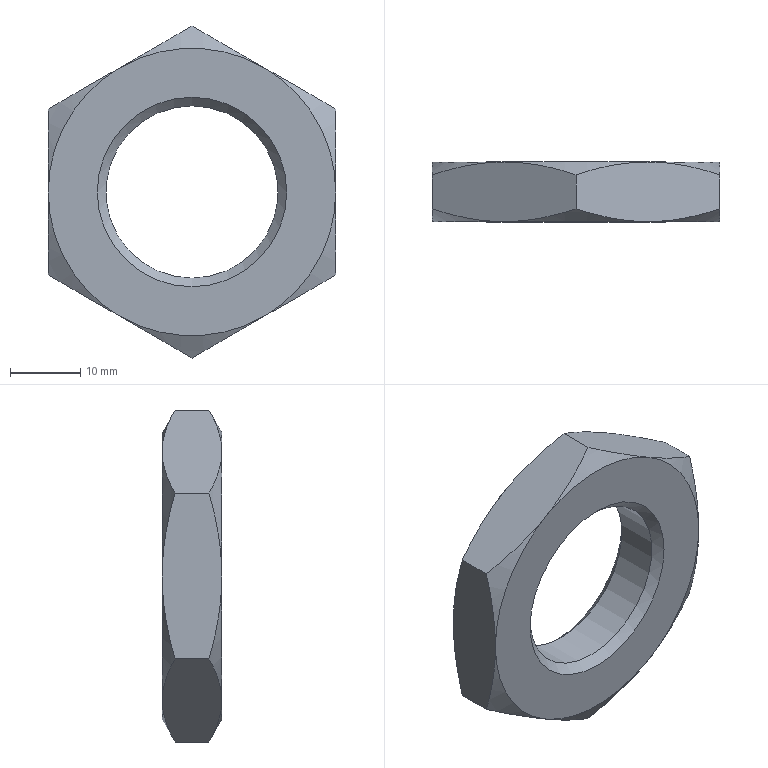Part | STEP file | Tube necking machine_id638_x_t | 1 solid | 23 faces | box 41 x 8.5 x 47.343 mm | volume 8073 mm3 | cone 14 | plane 8 | cylinder 1 | commonest cylinder face diameters 24.564 x1